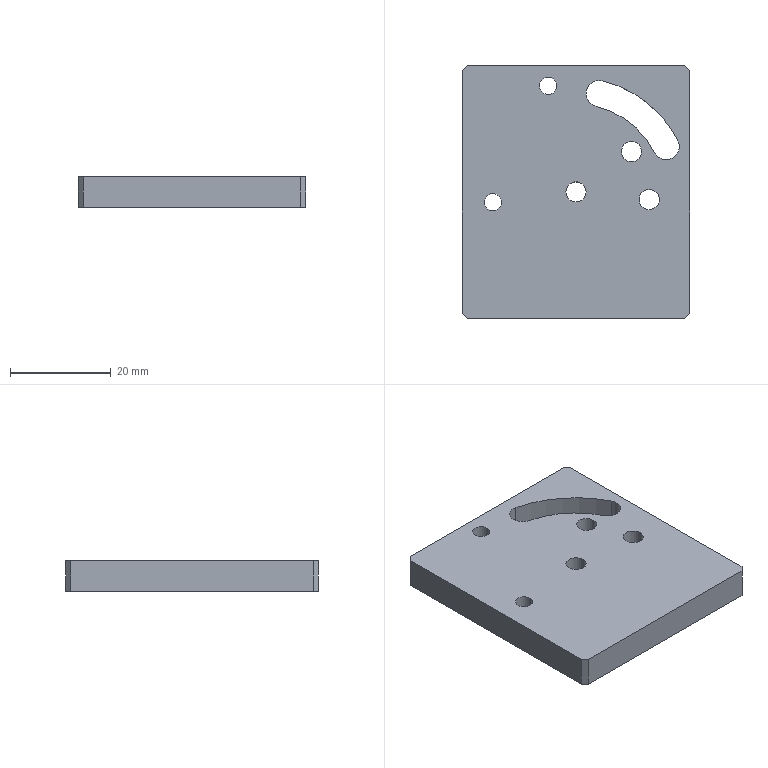Part | NX | features BREP 1 | 1 solid | 31 faces | box 45 x 50 x 6 mm | volume 12312 mm3 | cylinder 19 | plane 12 | commonest cylinder face diameters 4 x6 3.4 x4 6.5 x4 5.2 x3 34.8 x1 45.2 x1
STEP:
#1=CARTESIAN_POINT('',(12.5,-1.5,6.));
#2=VERTEX_POINT('',#1);
#3=CARTESIAN_POINT('',(16.5,-1.5,6.));
#4=VERTEX_POINT('',#3);
#5=CARTESIAN_POINT('',(14.5,-1.5,6.));
#6=DIRECTION('',(0.,0.,1.));
#7=DIRECTION('',(1.,0.,0.));
#8=AXIS2_PLACEMENT_3D('',#5,#6,#7);
#9=CIRCLE('',#8,2.);
#10=EDGE_CURVE('',#2,#4,#9,.T.);
#11=ORIENTED_EDGE('',*,*,#10,.T.);
#12=CARTESIAN_POINT('',(16.5,-1.5,0.));
#13=VERTEX_POINT('',#12);
#14=CARTESIAN_POINT('',(16.5,-1.5,10.));
#15=DIRECTION('',(0.,0.,-1.));
#16=VECTOR('',#15,1000.);
#17=LINE('',#14,#16);
#18=EDGE_CURVE('',#4,#13,#17,.T.);
#19=ORIENTED_EDGE('',*,*,#18,.T.);
#20=CARTESIAN_POINT('',(12.5,-1.5,0.));
#21=VERTEX_POINT('',#20);
#22=CARTESIAN_POINT('',(14.5,-1.5,0.));
#23=DIRECTION('',(0.,0.,-1.));
#24=DIRECTION('',(-1.,0.,0.));
#25=AXIS2_PLACEMENT_3D('',#22,#23,#24);
#26=CIRCLE('',#25,2.);
#27=EDGE_CURVE('',#13,#21,#26,.T.);
#28=ORIENTED_EDGE('',*,*,#27,.T.);
#29=CARTESIAN_POINT('',(12.5,-1.5,10.));
#30=DIRECTION('',(0.,0.,-1.));
#31=VECTOR('',#30,1000.);
#32=LINE('',#29,#31);
#33=EDGE_CURVE('',#2,#21,#32,.T.);
#34=ORIENTED_EDGE('',*,*,#33,.F.);
#35=EDGE_LOOP('',(#11,#19,#28,#34));
#36=FACE_BOUND('',#35,.T.);
#37=CARTESIAN_POINT('',(14.5,-1.5,10.));
#38=DIRECTION('',(0.,0.,-1.));
#39=DIRECTION('',(-1.,0.,0.));
#40=AXIS2_PLACEMENT_3D('',#37,#38,#39);
#41=CYLINDRICAL_SURFACE('',#40,2.);
#42=ADVANCED_FACE('',(#36),#41,.F.);
#43=CARTESIAN_POINT('',(9.,8.,6.));
#44=VERTEX_POINT('',#43);
#45=CARTESIAN_POINT('',(13.,8.,6.));
#46=VERTEX_POINT('',#45);
#47=CARTESIAN_POINT('',(11.,8.,6.));
#48=DIRECTION('',(0.,0.,1.));
#49=DIRECTION('',(1.,0.,0.));
#50=AXIS2_PLACEMENT_3D('',#47,#48,#49);
#51=CIRCLE('',#50,2.);
#52=EDGE_CURVE('',#44,#46,#51,.T.);
#53=ORIENTED_EDGE('',*,*,#52,.T.);
#54=CARTESIAN_POINT('',(13.,8.,0.));
#55=VERTEX_POINT('',#54);
#56=CARTESIAN_POINT('',(13.,8.,10.));
#57=DIRECTION('',(0.,0.,-1.));
#58=VECTOR('',#57,1000.);
#59=LINE('',#56,#58);
#60=EDGE_CURVE('',#46,#55,#59,.T.);
#61=ORIENTED_EDGE('',*,*,#60,.T.);
#62=CARTESIAN_POINT('',(9.,8.,0.));
#63=VERTEX_POINT('',#62);
#64=CARTESIAN_POINT('',(11.,8.,0.));
#65=DIRECTION('',(0.,0.,-1.));
#66=DIRECTION('',(-1.,0.,0.));
#67=AXIS2_PLACEMENT_3D('',#64,#65,#66);
#68=CIRCLE('',#67,2.);
#69=EDGE_CURVE('',#55,#63,#68,.T.);
#70=ORIENTED_EDGE('',*,*,#69,.T.);
#71=CARTESIAN_POINT('',(9.,8.,10.));
#72=DIRECTION('',(0.,0.,-1.));
#73=VECTOR('',#72,1000.);
#74=LINE('',#71,#73);
#75=EDGE_CURVE('',#44,#63,#74,.T.);
#76=ORIENTED_EDGE('',*,*,#75,.F.);
#77=EDGE_LOOP('',(#53,#61,#70,#76));
#78=FACE_BOUND('',#77,.T.);
#79=CARTESIAN_POINT('',(11.,8.,10.));
#80=DIRECTION('',(0.,0.,-1.));
#81=DIRECTION('',(-1.,0.,0.));
#82=AXIS2_PLACEMENT_3D('',#79,#80,#81);
#83=CYLINDRICAL_SURFACE('',#82,2.);
#84=ADVANCED_FACE('',(#78),#83,.F.);
#85=CARTESIAN_POINT('',(-13.25,-2.,3.5));
#86=VERTEX_POINT('',#85);
#87=CARTESIAN_POINT('',(-19.75,-2.,3.5));
#88=VERTEX_POINT('',#87);
#89=CARTESIAN_POINT('',(-16.5,-2.,3.5));
#90=DIRECTION('',(0.,0.,-1.));
#91=DIRECTION('',(-1.,0.,0.));
#92=AXIS2_PLACEMENT_3D('',#89,#90,#91);
#93=CIRCLE('',#92,3.25);
#94=EDGE_CURVE('',#86,#88,#93,.T.);
#95=ORIENTED_EDGE('',*,*,#94,.F.);
#96=CARTESIAN_POINT('',(-13.25,-2.,0.));
#97=VERTEX_POINT('',#96);
#98=CARTESIAN_POINT('',(-13.25,-2.,0.));
#99=DIRECTION('',(0.,0.,-1.));
#100=VECTOR('',#99,1000.);
#101=LINE('',#98,#100);
#102=EDGE_CURVE('',#86,#97,#101,.T.);
#103=ORIENTED_EDGE('',*,*,#102,.T.);
#104=CARTESIAN_POINT('',(-19.75,-2.,0.));
#105=VERTEX_POINT('',#104);
#106=CARTESIAN_POINT('',(-16.5,-2.,0.));
#107=DIRECTION('',(0.,0.,-1.));
#108=DIRECTION('',(-1.,0.,0.));
#109=AXIS2_PLACEMENT_3D('',#106,#107,#108);
#110=CIRCLE('',#109,3.25);
#111=EDGE_CURVE('',#97,#105,#110,.T.);
#112=ORIENTED_EDGE('',*,*,#111,.T.);
#113=CARTESIAN_POINT('',(-19.75,-2.,0.));
#114=DIRECTION('',(0.,0.,-1.));
#115=VECTOR('',#114,1000.);
#116=LINE('',#113,#115);
#117=EDGE_CURVE('',#88,#105,#116,.T.);
#118=ORIENTED_EDGE('',*,*,#117,.F.);
#119=EDGE_LOOP('',(#95,#103,#112,#118));
#120=FACE_BOUND('',#119,.T.);
#121=CARTESIAN_POINT('',(-16.5,-2.,0.));
#122=DIRECTION('',(0.,0.,-1.));
#123=DIRECTION('',(-1.,0.,0.));
#124=AXIS2_PLACEMENT_3D('',#121,#122,#123);
#125=CYLINDRICAL_SURFACE('',#124,3.25);
#126=ADVANCED_FACE('',(#120),#125,.F.);
#127=CARTESIAN_POINT('',(-14.8,-2.,6.));
#128=VERTEX_POINT('',#127);
#129=CARTESIAN_POINT('',(-18.2,-2.,6.));
#130=VERTEX_POINT('',#129);
#131=CARTESIAN_POINT('',(-16.5,-2.,6.));
#132=DIRECTION('',(0.,0.,-1.));
#133=DIRECTION('',(-1.,0.,0.));
#134=AXIS2_PLACEMENT_3D('',#131,#132,#133);
#135=CIRCLE('',#134,1.7);
#136=EDGE_CURVE('',#128,#130,#135,.T.);
#137=ORIENTED_EDGE('',*,*,#136,.F.);
#138=CARTESIAN_POINT('',(-14.8,-2.,3.5));
#139=VERTEX_POINT('',#138);
#140=CARTESIAN_POINT('',(-14.8,-2.,0.));
#141=DIRECTION('',(0.,0.,-1.));
#142=VECTOR('',#141,1000.);
#143=LINE('',#140,#142);
#144=EDGE_CURVE('',#128,#139,#143,.T.);
#145=ORIENTED_EDGE('',*,*,#144,.T.);
#146=CARTESIAN_POINT('',(-18.2,-2.,3.5));
#147=VERTEX_POINT('',#146);
#148=CARTESIAN_POINT('',(-16.5,-2.,3.5));
#149=DIRECTION('',(0.,0.,-1.));
#150=DIRECTION('',(-1.,0.,0.));
#151=AXIS2_PLACEMENT_3D('',#148,#149,#150);
#152=CIRCLE('',#151,1.7);
#153=EDGE_CURVE('',#139,#147,#152,.T.);
#154=ORIENTED_EDGE('',*,*,#153,.T.);
#155=CARTESIAN_POINT('',(-18.2,-2.,0.));
#156=DIRECTION('',(0.,0.,-1.));
#157=VECTOR('',#156,1000.);
#158=LINE('',#155,#157);
#159=EDGE_CURVE('',#130,#147,#158,.T.);
#160=ORIENTED_EDGE('',*,*,#159,.F.);
#161=EDGE_LOOP('',(#137,#145,#154,#160));
#162=FACE_BOUND('',#161,.T.);
#163=CARTESIAN_POINT('',(-16.5,-2.,0.));
#164=DIRECTION('',(0.,0.,-1.));
#165=DIRECTION('',(-1.,0.,0.));
#166=AXIS2_PLACEMENT_3D('',#163,#164,#165);
#167=CYLINDRICAL_SURFACE('',#166,1.7);
#168=ADVANCED_FACE('',(#162),#167,.F.);
#169=CARTESIAN_POINT('',(-2.25,21.,3.5));
#170=VERTEX_POINT('',#169);
#171=CARTESIAN_POINT('',(-8.75,21.,3.5));
#172=VERTEX_POINT('',#171);
#173=CARTESIAN_POINT('',(-5.5,21.,3.5));
#174=DIRECTION('',(0.,0.,-1.));
#175=DIRECTION('',(-1.,0.,0.));
#176=AXIS2_PLACEMENT_3D('',#173,#174,#175);
#177=CIRCLE('',#176,3.25);
#178=EDGE_CURVE('',#170,#172,#177,.T.);
#179=ORIENTED_EDGE('',*,*,#178,.F.);
#180=CARTESIAN_POINT('',(-2.25,21.,0.));
#181=VERTEX_POINT('',#180);
#182=CARTESIAN_POINT('',(-2.25,21.,0.));
#183=DIRECTION('',(0.,0.,-1.));
#184=VECTOR('',#183,1000.);
#185=LINE('',#182,#184);
#186=EDGE_CURVE('',#170,#181,#185,.T.);
#187=ORIENTED_EDGE('',*,*,#186,.T.);
#188=CARTESIAN_POINT('',(-8.75,21.,0.));
#189=VERTEX_POINT('',#188);
#190=CARTESIAN_POINT('',(-5.5,21.,0.));
#191=DIRECTION('',(0.,0.,-1.));
#192=DIRECTION('',(-1.,0.,0.));
#193=AXIS2_PLACEMENT_3D('',#190,#191,#192);
#194=CIRCLE('',#193,3.25);
#195=EDGE_CURVE('',#181,#189,#194,.T.);
#196=ORIENTED_EDGE('',*,*,#195,.T.);
#197=CARTESIAN_POINT('',(-8.75,21.,0.));
#198=DIRECTION('',(0.,0.,-1.));
#199=VECTOR('',#198,1000.);
#200=LINE('',#197,#199);
#201=EDGE_CURVE('',#172,#189,#200,.T.);
#202=ORIENTED_EDGE('',*,*,#201,.F.);
#203=EDGE_LOOP('',(#179,#187,#196,#202));
#204=FACE_BOUND('',#203,.T.);
#205=CARTESIAN_POINT('',(-5.5,21.,0.));
#206=DIRECTION('',(0.,0.,-1.));
#207=DIRECTION('',(-1.,0.,0.));
#208=AXIS2_PLACEMENT_3D('',#205,#206,#207);
#209=CYLINDRICAL_SURFACE('',#208,3.25);
#210=ADVANCED_FACE('',(#204),#209,.F.);
#211=CARTESIAN_POINT('',(-3.8,21.,6.));
#212=VERTEX_POINT('',#211);
#213=CARTESIAN_POINT('',(-7.2,21.,6.));
#214=VERTEX_POINT('',#213);
#215=CARTESIAN_POINT('',(-5.5,21.,6.));
#216=DIRECTION('',(0.,0.,-1.));
#217=DIRECTION('',(-1.,0.,0.));
#218=AXIS2_PLACEMENT_3D('',#215,#216,#217);
#219=CIRCLE('',#218,1.7);
#220=EDGE_CURVE('',#212,#214,#219,.T.);
#221=ORIENTED_EDGE('',*,*,#220,.F.);
#222=CARTESIAN_POINT('',(-3.8,21.,3.5));
#223=VERTEX_POINT('',#222);
#224=CARTESIAN_POINT('',(-3.8,21.,0.));
#225=DIRECTION('',(0.,0.,-1.));
#226=VECTOR('',#225,1000.);
#227=LINE('',#224,#226);
#228=EDGE_CURVE('',#212,#223,#227,.T.);
#229=ORIENTED_EDGE('',*,*,#228,.T.);
#230=CARTESIAN_POINT('',(-7.2,21.,3.5));
#231=VERTEX_POINT('',#230);
#232=CARTESIAN_POINT('',(-5.5,21.,3.5));
#233=DIRECTION('',(0.,0.,-1.));
#234=DIRECTION('',(-1.,0.,0.));
#235=AXIS2_PLACEMENT_3D('',#232,#233,#234);
#236=CIRCLE('',#235,1.7);
#237=EDGE_CURVE('',#223,#231,#236,.T.);
#238=ORIENTED_EDGE('',*,*,#237,.T.);
#239=CARTESIAN_POINT('',(-7.2,21.,0.));
#240=DIRECTION('',(0.,0.,-1.));
#241=VECTOR('',#240,1000.);
#242=LINE('',#239,#241);
#243=EDGE_CURVE('',#214,#231,#242,.T.);
#244=ORIENTED_EDGE('',*,*,#243,.F.);
#245=EDGE_LOOP('',(#221,#229,#238,#244));
#246=FACE_BOUND('',#245,.T.);
#247=CARTESIAN_POINT('',(-5.5,21.,0.));
#248=DIRECTION('',(0.,0.,-1.));
#249=DIRECTION('',(-1.,0.,0.));
#250=AXIS2_PLACEMENT_3D('',#247,#248,#249);
#251=CYLINDRICAL_SURFACE('',#250,1.7);
#252=ADVANCED_FACE('',(#246),#251,.F.);
#253=CARTESIAN_POINT('',(5.182,21.998,6.));
#254=VERTEX_POINT('',#253);
#255=CARTESIAN_POINT('',(1.986,19.467,6.));
#256=VERTEX_POINT('',#255);
#257=CARTESIAN_POINT('',(4.586,19.467,6.));
#258=DIRECTION('',(0.,0.,1.));
#259=DIRECTION('',(1.,0.,0.));
#260=AXIS2_PLACEMENT_3D('',#257,#258,#259);
#261=CIRCLE('',#260,2.6);
#262=EDGE_CURVE('',#254,#256,#261,.T.);
#263=ORIENTED_EDGE('',*,*,#262,.T.);
#264=CARTESIAN_POINT('',(1.986,19.467,0.));
#265=VERTEX_POINT('',#264);
#266=CARTESIAN_POINT('',(1.986,19.467,10.));
#267=DIRECTION('',(0.,0.,-1.));
#268=VECTOR('',#267,1000.);
#269=LINE('',#266,#268);
#270=EDGE_CURVE('',#256,#265,#269,.T.);
#271=ORIENTED_EDGE('',*,*,#270,.T.);
#272=CARTESIAN_POINT('',(5.182,21.998,0.));
#273=VERTEX_POINT('',#272);
#274=CARTESIAN_POINT('',(4.586,19.467,0.));
#275=DIRECTION('',(0.,0.,-1.));
#276=DIRECTION('',(-1.,0.,0.));
#277=AXIS2_PLACEMENT_3D('',#274,#275,#276);
#278=CIRCLE('',#277,2.6);
#279=EDGE_CURVE('',#265,#273,#278,.T.);
#280=ORIENTED_EDGE('',*,*,#279,.T.);
#281=CARTESIAN_POINT('',(5.182,21.998,10.));
#282=DIRECTION('',(0.,0.,-1.));
#283=VECTOR('',#282,1000.);
#284=LINE('',#281,#283);
#285=EDGE_CURVE('',#254,#273,#284,.T.);
#286=ORIENTED_EDGE('',*,*,#285,.F.);
#287=EDGE_LOOP('',(#263,#271,#280,#286));
#288=FACE_BOUND('',#287,.T.);
#289=CARTESIAN_POINT('',(4.586,19.467,10.));
#290=DIRECTION('',(0.,0.,-1.));
#291=DIRECTION('',(-1.,0.,0.));
#292=AXIS2_PLACEMENT_3D('',#289,#290,#291);
#293=CYLINDRICAL_SURFACE('',#292,2.6);
#294=ADVANCED_FACE('',(#288),#293,.F.);
#295=CARTESIAN_POINT('',(-2.,0.,6.));
#296=VERTEX_POINT('',#295);
#297=CARTESIAN_POINT('',(2.,0.,6.));
#298=VERTEX_POINT('',#297);
#299=CARTESIAN_POINT('',(0.,0.,6.));
#300=DIRECTION('',(0.,0.,1.));
#301=DIRECTION('',(1.,0.,0.));
#302=AXIS2_PLACEMENT_3D('',#299,#300,#301);
#303=CIRCLE('',#302,2.);
#304=EDGE_CURVE('',#296,#298,#303,.T.);
#305=ORIENTED_EDGE('',*,*,#304,.T.);
#306=CARTESIAN_POINT('',(2.,0.,0.));
#307=VERTEX_POINT('',#306);
#308=CARTESIAN_POINT('',(2.,0.,10.));
#309=DIRECTION('',(0.,0.,-1.));
#310=VECTOR('',#309,1000.);
#311=LINE('',#308,#310);
#312=EDGE_CURVE('',#298,#307,#311,.T.);
#313=ORIENTED_EDGE('',*,*,#312,.T.);
#314=CARTESIAN_POINT('',(-2.,0.,0.));
#315=VERTEX_POINT('',#314);
#316=CARTESIAN_POINT('',(0.,0.,0.));
#317=DIRECTION('',(0.,0.,-1.));
#318=DIRECTION('',(-1.,0.,0.));
#319=AXIS2_PLACEMENT_3D('',#316,#317,#318);
#320=CIRCLE('',#319,2.);
#321=EDGE_CURVE('',#307,#315,#320,.T.);
#322=ORIENTED_EDGE('',*,*,#321,.T.);
#323=CARTESIAN_POINT('',(-2.,0.,10.));
#324=DIRECTION('',(0.,0.,-1.));
#325=VECTOR('',#324,1000.);
#326=LINE('',#323,#325);
#327=EDGE_CURVE('',#296,#315,#326,.T.);
#328=ORIENTED_EDGE('',*,*,#327,.F.);
#329=EDGE_LOOP('',(#305,#313,#322,#328));
#330=FACE_BOUND('',#329,.T.);
#331=CARTESIAN_POINT('',(0.,0.,10.));
#332=DIRECTION('',(0.,0.,-1.));
#333=DIRECTION('',(-1.,0.,0.));
#334=AXIS2_PLACEMENT_3D('',#331,#332,#333);
#335=CYLINDRICAL_SURFACE('',#334,2.);
#336=ADVANCED_FACE('',(#330),#335,.F.);
#337=CARTESIAN_POINT('',(22.5,-24.,6.));
#338=VERTEX_POINT('',#337);
#339=CARTESIAN_POINT('',(22.5,24.,6.));
#340=VERTEX_POINT('',#339);
#341=CARTESIAN_POINT('',(22.5,25.,6.));
#342=DIRECTION('',(0.,1.,0.));
#343=VECTOR('',#342,1000.);
#344=LINE('',#341,#343);
#345=EDGE_CURVE('',#338,#340,#344,.T.);
#346=ORIENTED_EDGE('',*,*,#345,.F.);
#347=CARTESIAN_POINT('',(22.5,-24.,0.));
#348=VERTEX_POINT('',#347);
#349=CARTESIAN_POINT('',(22.5,-24.,6.));
#350=DIRECTION('',(0.,0.,-1.));
#351=VECTOR('',#350,1000.);
#352=LINE('',#349,#351);
#353=EDGE_CURVE('',#338,#348,#352,.T.);
#354=ORIENTED_EDGE('',*,*,#353,.T.);
#355=CARTESIAN_POINT('',(22.5,24.,0.));
#356=VERTEX_POINT('',#355);
#357=CARTESIAN_POINT('',(22.5,25.,0.));
#358=DIRECTION('',(0.,1.,0.));
#359=VECTOR('',#358,1000.);
#360=LINE('',#357,#359);
#361=EDGE_CURVE('',#348,#356,#360,.T.);
#362=ORIENTED_EDGE('',*,*,#361,.T.);
#363=CARTESIAN_POINT('',(22.5,24.,6.));
#364=DIRECTION('',(0.,0.,1.));
#365=VECTOR('',#364,1000.);
#366=LINE('',#363,#365);
#367=EDGE_CURVE('',#356,#340,#366,.T.);
#368=ORIENTED_EDGE('',*,*,#367,.T.);
#369=EDGE_LOOP('',(#346,#354,#362,#368));
#370=FACE_BOUND('',#369,.T.);
#371=CARTESIAN_POINT('',(22.5,25.,6.));
#372=DIRECTION('',(-1.,0.,0.));
#373=DIRECTION('',(0.,1.,0.));
#374=AXIS2_PLACEMENT_3D('',#371,#372,#373);
#375=PLANE('',#374);
#376=ADVANCED_FACE('',(#370),#375,.F.);
#377=CARTESIAN_POINT('',(21.5,25.,0.));
#378=VERTEX_POINT('',#377);
#379=CARTESIAN_POINT('',(-21.5,25.,0.));
#380=VERTEX_POINT('',#379);
#381=CARTESIAN_POINT('',(-22.5,25.,0.));
#382=DIRECTION('',(-1.,0.,0.));
#383=VECTOR('',#382,1000.);
#384=LINE('',#381,#383);
#385=EDGE_CURVE('',#378,#380,#384,.T.);
#386=ORIENTED_EDGE('',*,*,#385,.T.);
#387=CARTESIAN_POINT('',(-21.5,25.,6.));
#388=VERTEX_POINT('',#387);
#389=CARTESIAN_POINT('',(-21.5,25.,6.));
#390=DIRECTION('',(0.,0.,1.));
#391=VECTOR('',#390,1000.);
#392=LINE('',#389,#391);
#393=EDGE_CURVE('',#380,#388,#392,.T.);
#394=ORIENTED_EDGE('',*,*,#393,.T.);
#395=CARTESIAN_POINT('',(21.5,25.,6.));
#396=VERTEX_POINT('',#395);
#397=CARTESIAN_POINT('',(-22.5,25.,6.));
#398=DIRECTION('',(-1.,0.,0.));
#399=VECTOR('',#398,1000.);
#400=LINE('',#397,#399);
#401=EDGE_CURVE('',#396,#388,#400,.T.);
#402=ORIENTED_EDGE('',*,*,#401,.F.);
#403=CARTESIAN_POINT('',(21.5,25.,6.));
#404=DIRECTION('',(0.,0.,-1.));
#405=VECTOR('',#404,1000.);
#406=LINE('',#403,#405);
#407=EDGE_CURVE('',#396,#378,#406,.T.);
#408=ORIENTED_EDGE('',*,*,#407,.T.);
#409=EDGE_LOOP('',(#386,#394,#402,#408));
#410=FACE_BOUND('',#409,.T.);
#411=CARTESIAN_POINT('',(-22.5,25.,6.));
#412=DIRECTION('',(0.,-1.,0.));
#413=DIRECTION('',(0.,0.,-1.));
#414=AXIS2_PLACEMENT_3D('',#411,#412,#413);
#415=PLANE('',#414);
#416=ADVANCED_FACE('',(#410),#415,.F.);
#417=CARTESIAN_POINT('',(-22.5,24.,0.));
#418=VERTEX_POINT('',#417);
#419=CARTESIAN_POINT('',(-22.5,-24.,0.));
#420=VERTEX_POINT('',#419);
#421=CARTESIAN_POINT('',(-22.5,25.,0.));
#422=DIRECTION('',(0.,-1.,0.));
#423=VECTOR('',#422,1000.);
#424=LINE('',#421,#423);
#425=EDGE_CURVE('',#418,#420,#424,.T.);
#426=ORIENTED_EDGE('',*,*,#425,.T.);
#427=CARTESIAN_POINT('',(-22.5,-24.,6.));
#428=VERTEX_POINT('',#427);
#429=CARTESIAN_POINT('',(-22.5,-24.,6.));
#430=DIRECTION('',(0.,0.,1.));
#431=VECTOR('',#430,1000.);
#432=LINE('',#429,#431);
#433=EDGE_CURVE('',#420,#428,#432,.T.);
#434=ORIENTED_EDGE('',*,*,#433,.T.);
#435=CARTESIAN_POINT('',(-22.5,24.,6.));
#436=VERTEX_POINT('',#435);
#437=CARTESIAN_POINT('',(-22.5,25.,6.));
#438=DIRECTION('',(0.,-1.,0.));
#439=VECTOR('',#438,1000.);
#440=LINE('',#437,#439);
#441=EDGE_CURVE('',#436,#428,#440,.T.);
#442=ORIENTED_EDGE('',*,*,#441,.F.);
#443=CARTESIAN_POINT('',(-22.5,24.,6.));
#444=DIRECTION('',(0.,0.,-1.));
#445=VECTOR('',#444,1000.);
#446=LINE('',#443,#445);
#447=EDGE_CURVE('',#436,#418,#446,.T.);
#448=ORIENTED_EDGE('',*,*,#447,.T.);
#449=EDGE_LOOP('',(#426,#434,#442,#448));
#450=FACE_BOUND('',#449,.T.);
#451=CARTESIAN_POINT('',(-22.5,25.,6.));
#452=DIRECTION('',(1.,0.,0.));
#453=DIRECTION('',(0.,1.,0.));
#454=AXIS2_PLACEMENT_3D('',#451,#452,#453);
#455=PLANE('',#454);
#456=ADVANCED_FACE('',(#450),#455,.F.);
#457=CARTESIAN_POINT('',(-21.5,-25.,6.));
#458=VERTEX_POINT('',#457);
#459=CARTESIAN_POINT('',(21.5,-25.,6.));
#460=VERTEX_POINT('',#459);
#461=CARTESIAN_POINT('',(-22.5,-25.,6.));
#462=DIRECTION('',(1.,0.,0.));
#463=VECTOR('',#462,1000.);
#464=LINE('',#461,#463);
#465=EDGE_CURVE('',#458,#460,#464,.T.);
#466=ORIENTED_EDGE('',*,*,#465,.F.);
#467=CARTESIAN_POINT('',(-21.5,-25.,0.));
#468=VERTEX_POINT('',#467);
#469=CARTESIAN_POINT('',(-21.5,-25.,6.));
#470=DIRECTION('',(0.,0.,-1.));
#471=VECTOR('',#470,1000.);
#472=LINE('',#469,#471);
#473=EDGE_CURVE('',#458,#468,#472,.T.);
#474=ORIENTED_EDGE('',*,*,#473,.T.);
#475=CARTESIAN_POINT('',(21.5,-25.,0.));
#476=VERTEX_POINT('',#475);
#477=CARTESIAN_POINT('',(-22.5,-25.,0.));
#478=DIRECTION('',(1.,0.,0.));
#479=VECTOR('',#478,1000.);
#480=LINE('',#477,#479);
#481=EDGE_CURVE('',#468,#476,#480,.T.);
#482=ORIENTED_EDGE('',*,*,#481,.T.);
#483=CARTESIAN_POINT('',(21.5,-25.,6.));
#484=DIRECTION('',(0.,0.,1.));
#485=VECTOR('',#484,1000.);
#486=LINE('',#483,#485);
#487=EDGE_CURVE('',#476,#460,#486,.T.);
#488=ORIENTED_EDGE('',*,*,#487,.T.);
#489=EDGE_LOOP('',(#466,#474,#482,#488));
#490=FACE_BOUND('',#489,.T.);
#491=CARTESIAN_POINT('',(-22.5,-25.,6.));
#492=DIRECTION('',(0.,1.,0.));
#493=DIRECTION('',(1.,0.,0.));
#494=AXIS2_PLACEMENT_3D('',#491,#492,#493);
#495=PLANE('',#494);
#496=ADVANCED_FACE('',(#490),#495,.F.);
#497=ORIENTED_EDGE('',*,*,#441,.T.);
#498=CARTESIAN_POINT('',(-23.25,-23.25,6.));
#499=DIRECTION('',(0.7071,-0.7071,0.));
#500=VECTOR('',#499,1000.);
#501=LINE('',#498,#500);
#502=EDGE_CURVE('',#428,#458,#501,.T.);
#503=ORIENTED_EDGE('',*,*,#502,.T.);
#504=ORIENTED_EDGE('',*,*,#465,.T.);
#505=CARTESIAN_POINT('',(23.25,-23.25,6.));
#506=DIRECTION('',(0.7071,0.7071,0.));
#507=VECTOR('',#506,1000.);
#508=LINE('',#505,#507);
#509=EDGE_CURVE('',#460,#338,#508,.T.);
#510=ORIENTED_EDGE('',*,*,#509,.T.);
#511=ORIENTED_EDGE('',*,*,#345,.T.);
#512=CARTESIAN_POINT('',(23.25,23.25,6.));
#513=DIRECTION('',(-0.7071,0.7071,0.));
#514=VECTOR('',#513,1000.);
#515=LINE('',#512,#514);
#516=EDGE_CURVE('',#340,#396,#515,.T.);
#517=ORIENTED_EDGE('',*,*,#516,.T.);
#518=ORIENTED_EDGE('',*,*,#401,.T.);
#519=CARTESIAN_POINT('',(-23.25,23.25,6.));
#520=DIRECTION('',(-0.7071,-0.7071,0.));
#521=VECTOR('',#520,1000.);
#522=LINE('',#519,#521);
#523=EDGE_CURVE('',#388,#436,#522,.T.);
#524=ORIENTED_EDGE('',*,*,#523,.T.);
#525=EDGE_LOOP('',(#497,#503,#504,#510,#511,#517,#518,#524));
#526=FACE_BOUND('',#525,.T.);
#527=ORIENTED_EDGE('',*,*,#10,.F.);
#528=CARTESIAN_POINT('',(14.5,-1.5,6.));
#529=DIRECTION('',(0.,0.,1.));
#530=DIRECTION('',(1.,0.,0.));
#531=AXIS2_PLACEMENT_3D('',#528,#529,#530);
#532=CIRCLE('',#531,2.);
#533=EDGE_CURVE('',#4,#2,#532,.T.);
#534=ORIENTED_EDGE('',*,*,#533,.F.);
#535=EDGE_LOOP('',(#527,#534));
#536=FACE_BOUND('',#535,.T.);
#537=ORIENTED_EDGE('',*,*,#52,.F.);
#538=CARTESIAN_POINT('',(11.,8.,6.));
#539=DIRECTION('',(0.,0.,1.));
#540=DIRECTION('',(1.,0.,0.));
#541=AXIS2_PLACEMENT_3D('',#538,#539,#540);
#542=CIRCLE('',#541,2.);
#543=EDGE_CURVE('',#46,#44,#542,.T.);
#544=ORIENTED_EDGE('',*,*,#543,.F.);
#545=EDGE_LOOP('',(#537,#544));
#546=FACE_BOUND('',#545,.T.);
#547=CARTESIAN_POINT('',(-16.5,-2.,6.));
#548=DIRECTION('',(0.,0.,-1.));
#549=DIRECTION('',(-1.,0.,0.));
#550=AXIS2_PLACEMENT_3D('',#547,#548,#549);
#551=CIRCLE('',#550,1.7);
#552=EDGE_CURVE('',#130,#128,#551,.T.);
#553=ORIENTED_EDGE('',*,*,#552,.T.);
#554=ORIENTED_EDGE('',*,*,#136,.T.);
#555=EDGE_LOOP('',(#553,#554));
#556=FACE_BOUND('',#555,.T.);
#557=CARTESIAN_POINT('',(-5.5,21.,6.));
#558=DIRECTION('',(0.,0.,-1.));
#559=DIRECTION('',(-1.,0.,0.));
#560=AXIS2_PLACEMENT_3D('',#557,#558,#559);
#561=CIRCLE('',#560,1.7);
#562=EDGE_CURVE('',#214,#212,#561,.T.);
#563=ORIENTED_EDGE('',*,*,#562,.T.);
#564=ORIENTED_EDGE('',*,*,#220,.T.);
#565=EDGE_LOOP('',(#563,#564));
#566=FACE_BOUND('',#565,.T.);
#567=ORIENTED_EDGE('',*,*,#262,.F.);
#568=CARTESIAN_POINT('',(20.182,10.17,6.));
#569=VERTEX_POINT('',#568);
#570=CARTESIAN_POINT('',(0.,0.,6.));
#571=DIRECTION('',(0.,0.,1.));
#572=DIRECTION('',(1.,0.,0.));
#573=AXIS2_PLACEMENT_3D('',#570,#571,#572);
#574=CIRCLE('',#573,22.6);
#575=EDGE_CURVE('',#569,#254,#574,.T.);
#576=ORIENTED_EDGE('',*,*,#575,.F.);
#577=CARTESIAN_POINT('',(15.539,7.83,6.));
#578=VERTEX_POINT('',#577);
#579=CARTESIAN_POINT('',(17.861,9.,6.));
#580=DIRECTION('',(0.,0.,1.));
#581=DIRECTION('',(1.,0.,0.));
#582=AXIS2_PLACEMENT_3D('',#579,#580,#581);
#583=CIRCLE('',#582,2.6);
#584=EDGE_CURVE('',#578,#569,#583,.T.);
#585=ORIENTED_EDGE('',*,*,#584,.F.);
#586=CARTESIAN_POINT('',(3.99,16.936,6.));
#587=VERTEX_POINT('',#586);
#588=CARTESIAN_POINT('',(0.,0.,6.));
#589=DIRECTION('',(0.,0.,-1.));
#590=DIRECTION('',(1.,0.,0.));
#591=AXIS2_PLACEMENT_3D('',#588,#589,#590);
#592=CIRCLE('',#591,17.4);
#593=EDGE_CURVE('',#587,#578,#592,.T.);
#594=ORIENTED_EDGE('',*,*,#593,.F.);
#595=CARTESIAN_POINT('',(4.586,19.467,6.));
#596=DIRECTION('',(0.,0.,1.));
#597=DIRECTION('',(1.,0.,0.));
#598=AXIS2_PLACEMENT_3D('',#595,#596,#597);
#599=CIRCLE('',#598,2.6);
#600=EDGE_CURVE('',#256,#587,#599,.T.);
#601=ORIENTED_EDGE('',*,*,#600,.F.);
#602=EDGE_LOOP('',(#567,#576,#585,#594,#601));
#603=FACE_BOUND('',#602,.T.);
#604=ORIENTED_EDGE('',*,*,#304,.F.);
#605=CARTESIAN_POINT('',(0.,0.,6.));
#606=DIRECTION('',(0.,0.,1.));
#607=DIRECTION('',(1.,0.,0.));
#608=AXIS2_PLACEMENT_3D('',#605,#606,#607);
#609=CIRCLE('',#608,2.);
#610=EDGE_CURVE('',#298,#296,#609,.T.);
#611=ORIENTED_EDGE('',*,*,#610,.F.);
#612=EDGE_LOOP('',(#604,#611));
#613=FACE_BOUND('',#612,.T.);
#614=CARTESIAN_POINT('',(0.,0.,6.));
#615=DIRECTION('',(0.,0.,1.));
#616=DIRECTION('',(1.,0.,0.));
#617=AXIS2_PLACEMENT_3D('',#614,#615,#616);
#618=PLANE('',#617);
#619=ADVANCED_FACE('',(#526,#536,#546,#556,#566,#603,#613),#618,.T.);
#620=ORIENTED_EDGE('',*,*,#481,.F.);
#621=CARTESIAN_POINT('',(-21.5,-25.,0.));
#622=DIRECTION('',(-0.7071,0.7071,0.));
#623=VECTOR('',#622,1000.);
#624=LINE('',#621,#623);
#625=EDGE_CURVE('',#468,#420,#624,.T.);
#626=ORIENTED_EDGE('',*,*,#625,.T.);
#627=ORIENTED_EDGE('',*,*,#425,.F.);
#628=CARTESIAN_POINT('',(-22.5,24.,0.));
#629=DIRECTION('',(0.7071,0.7071,0.));
#630=VECTOR('',#629,1000.);
#631=LINE('',#628,#630);
#632=EDGE_CURVE('',#418,#380,#631,.T.);
#633=ORIENTED_EDGE('',*,*,#632,.T.);
#634=ORIENTED_EDGE('',*,*,#385,.F.);
#635=CARTESIAN_POINT('',(21.5,25.,0.));
#636=DIRECTION('',(0.7071,-0.7071,0.));
#637=VECTOR('',#636,1000.);
#638=LINE('',#635,#637);
#639=EDGE_CURVE('',#378,#356,#638,.T.);
#640=ORIENTED_EDGE('',*,*,#639,.T.);
#641=ORIENTED_EDGE('',*,*,#361,.F.);
#642=CARTESIAN_POINT('',(22.5,-24.,0.));
#643=DIRECTION('',(-0.7071,-0.7071,0.));
#644=VECTOR('',#643,1000.);
#645=LINE('',#642,#644);
#646=EDGE_CURVE('',#348,#476,#645,.T.);
#647=ORIENTED_EDGE('',*,*,#646,.T.);
#648=EDGE_LOOP('',(#620,#626,#627,#633,#634,#640,#641,#647));
#649=FACE_BOUND('',#648,.T.);
#650=CARTESIAN_POINT('',(14.5,-1.5,0.));
#651=DIRECTION('',(0.,0.,-1.));
#652=DIRECTION('',(-1.,0.,0.));
#653=AXIS2_PLACEMENT_3D('',#650,#651,#652);
#654=CIRCLE('',#653,2.);
#655=EDGE_CURVE('',#21,#13,#654,.T.);
#656=ORIENTED_EDGE('',*,*,#655,.F.);
#657=ORIENTED_EDGE('',*,*,#27,.F.);
#658=EDGE_LOOP('',(#656,#657));
#659=FACE_BOUND('',#658,.T.);
#660=CARTESIAN_POINT('',(11.,8.,0.));
#661=DIRECTION('',(0.,0.,-1.));
#662=DIRECTION('',(-1.,0.,0.));
#663=AXIS2_PLACEMENT_3D('',#660,#661,#662);
#664=CIRCLE('',#663,2.);
#665=EDGE_CURVE('',#63,#55,#664,.T.);
#666=ORIENTED_EDGE('',*,*,#665,.F.);
#667=ORIENTED_EDGE('',*,*,#69,.F.);
#668=EDGE_LOOP('',(#666,#667));
#669=FACE_BOUND('',#668,.T.);
#670=CARTESIAN_POINT('',(-16.5,-2.,0.));
#671=DIRECTION('',(0.,0.,-1.));
#672=DIRECTION('',(-1.,0.,0.));
#673=AXIS2_PLACEMENT_3D('',#670,#671,#672);
#674=CIRCLE('',#673,3.25);
#675=EDGE_CURVE('',#105,#97,#674,.T.);
#676=ORIENTED_EDGE('',*,*,#675,.F.);
#677=ORIENTED_EDGE('',*,*,#111,.F.);
#678=EDGE_LOOP('',(#676,#677));
#679=FACE_BOUND('',#678,.T.);
#680=CARTESIAN_POINT('',(-5.5,21.,0.));
#681=DIRECTION('',(0.,0.,-1.));
#682=DIRECTION('',(-1.,0.,0.));
#683=AXIS2_PLACEMENT_3D('',#680,#681,#682);
#684=CIRCLE('',#683,3.25);
#685=EDGE_CURVE('',#189,#181,#684,.T.);
#686=ORIENTED_EDGE('',*,*,#685,.F.);
#687=ORIENTED_EDGE('',*,*,#195,.F.);
#688=EDGE_LOOP('',(#686,#687));
#689=FACE_BOUND('',#688,.T.);
#690=CARTESIAN_POINT('',(20.182,10.17,0.));
#691=VERTEX_POINT('',#690);
#692=CARTESIAN_POINT('',(0.,0.,0.));
#693=DIRECTION('',(0.,0.,-1.));
#694=DIRECTION('',(-1.,0.,0.));
#695=AXIS2_PLACEMENT_3D('',#692,#693,#694);
#696=CIRCLE('',#695,22.6);
#697=EDGE_CURVE('',#273,#691,#696,.T.);
#698=ORIENTED_EDGE('',*,*,#697,.F.);
#699=ORIENTED_EDGE('',*,*,#279,.F.);
#700=CARTESIAN_POINT('',(3.99,16.936,0.));
#701=VERTEX_POINT('',#700);
#702=CARTESIAN_POINT('',(4.586,19.467,0.));
#703=DIRECTION('',(0.,0.,-1.));
#704=DIRECTION('',(-1.,0.,0.));
#705=AXIS2_PLACEMENT_3D('',#702,#703,#704);
#706=CIRCLE('',#705,2.6);
#707=EDGE_CURVE('',#701,#265,#706,.T.);
#708=ORIENTED_EDGE('',*,*,#707,.F.);
#709=CARTESIAN_POINT('',(15.539,7.83,0.));
#710=VERTEX_POINT('',#709);
#711=CARTESIAN_POINT('',(0.,0.,0.));
#712=DIRECTION('',(0.,0.,1.));
#713=DIRECTION('',(-1.,0.,0.));
#714=AXIS2_PLACEMENT_3D('',#711,#712,#713);
#715=CIRCLE('',#714,17.4);
#716=EDGE_CURVE('',#710,#701,#715,.T.);
#717=ORIENTED_EDGE('',*,*,#716,.F.);
#718=CARTESIAN_POINT('',(17.861,9.,0.));
#719=DIRECTION('',(0.,0.,-1.));
#720=DIRECTION('',(-1.,0.,0.));
#721=AXIS2_PLACEMENT_3D('',#718,#719,#720);
#722=CIRCLE('',#721,2.6);
#723=EDGE_CURVE('',#691,#710,#722,.T.);
#724=ORIENTED_EDGE('',*,*,#723,.F.);
#725=EDGE_LOOP('',(#698,#699,#708,#717,#724));
#726=FACE_BOUND('',#725,.T.);
#727=CARTESIAN_POINT('',(0.,0.,0.));
#728=DIRECTION('',(0.,0.,-1.));
#729=DIRECTION('',(-1.,0.,0.));
#730=AXIS2_PLACEMENT_3D('',#727,#728,#729);
#731=CIRCLE('',#730,2.);
#732=EDGE_CURVE('',#315,#307,#731,.T.);
#733=ORIENTED_EDGE('',*,*,#732,.F.);
#734=ORIENTED_EDGE('',*,*,#321,.F.);
#735=EDGE_LOOP('',(#733,#734));
#736=FACE_BOUND('',#735,.T.);
#737=CARTESIAN_POINT('',(0.,0.,0.));
#738=DIRECTION('',(0.,0.,1.));
#739=DIRECTION('',(1.,0.,0.));
#740=AXIS2_PLACEMENT_3D('',#737,#738,#739);
#741=PLANE('',#740);
#742=ADVANCED_FACE('',(#649,#659,#669,#679,#689,#726,#736),#741,.F.);
#743=ORIENTED_EDGE('',*,*,#502,.F.);
#744=ORIENTED_EDGE('',*,*,#433,.F.);
#745=ORIENTED_EDGE('',*,*,#625,.F.);
#746=ORIENTED_EDGE('',*,*,#473,.F.);
#747=EDGE_LOOP('',(#743,#744,#745,#746));
#748=FACE_BOUND('',#747,.T.);
#749=CARTESIAN_POINT('',(-21.5,-25.,6.));
#750=DIRECTION('',(0.7071,0.7071,0.));
#751=DIRECTION('',(0.,0.,-1.));
#752=AXIS2_PLACEMENT_3D('',#749,#750,#751);
#753=PLANE('',#752);
#754=ADVANCED_FACE('',(#748),#753,.F.);
#755=ORIENTED_EDGE('',*,*,#509,.F.);
#756=ORIENTED_EDGE('',*,*,#487,.F.);
#757=ORIENTED_EDGE('',*,*,#646,.F.);
#758=ORIENTED_EDGE('',*,*,#353,.F.);
#759=EDGE_LOOP('',(#755,#756,#757,#758));
#760=FACE_BOUND('',#759,.T.);
#761=CARTESIAN_POINT('',(22.5,-24.,6.));
#762=DIRECTION('',(-0.7071,0.7071,0.));
#763=DIRECTION('',(0.,0.,1.));
#764=AXIS2_PLACEMENT_3D('',#761,#762,#763);
#765=PLANE('',#764);
#766=ADVANCED_FACE('',(#760),#765,.F.);
#767=ORIENTED_EDGE('',*,*,#523,.F.);
#768=ORIENTED_EDGE('',*,*,#393,.F.);
#769=ORIENTED_EDGE('',*,*,#632,.F.);
#770=ORIENTED_EDGE('',*,*,#447,.F.);
#771=EDGE_LOOP('',(#767,#768,#769,#770));
#772=FACE_BOUND('',#771,.T.);
#773=CARTESIAN_POINT('',(-22.5,24.,6.));
#774=DIRECTION('',(0.7071,-0.7071,0.));
#775=DIRECTION('',(0.,0.,-1.));
#776=AXIS2_PLACEMENT_3D('',#773,#774,#775);
#777=PLANE('',#776);
#778=ADVANCED_FACE('',(#772),#777,.F.);
#779=ORIENTED_EDGE('',*,*,#516,.F.);
#780=ORIENTED_EDGE('',*,*,#367,.F.);
#781=ORIENTED_EDGE('',*,*,#639,.F.);
#782=ORIENTED_EDGE('',*,*,#407,.F.);
#783=EDGE_LOOP('',(#779,#780,#781,#782));
#784=FACE_BOUND('',#783,.T.);
#785=CARTESIAN_POINT('',(21.5,25.,6.));
#786=DIRECTION('',(-0.7071,-0.7071,0.));
#787=DIRECTION('',(-0.7071,0.7071,0.));
#788=AXIS2_PLACEMENT_3D('',#785,#786,#787);
#789=PLANE('',#788);
#790=ADVANCED_FACE('',(#784),#789,.F.);
#791=ORIENTED_EDGE('',*,*,#312,.F.);
#792=ORIENTED_EDGE('',*,*,#610,.T.);
#793=ORIENTED_EDGE('',*,*,#327,.T.);
#794=ORIENTED_EDGE('',*,*,#732,.T.);
#795=EDGE_LOOP('',(#791,#792,#793,#794));
#796=FACE_BOUND('',#795,.T.);
#797=CARTESIAN_POINT('',(0.,0.,10.));
#798=DIRECTION('',(0.,0.,-1.));
#799=DIRECTION('',(-1.,0.,0.));
#800=AXIS2_PLACEMENT_3D('',#797,#798,#799);
#801=CYLINDRICAL_SURFACE('',#800,2.);
#802=ADVANCED_FACE('',(#796),#801,.F.);
#803=ORIENTED_EDGE('',*,*,#270,.F.);
#804=ORIENTED_EDGE('',*,*,#600,.T.);
#805=CARTESIAN_POINT('',(3.99,16.936,10.));
#806=DIRECTION('',(0.,0.,-1.));
#807=VECTOR('',#806,1000.);
#808=LINE('',#805,#807);
#809=EDGE_CURVE('',#587,#701,#808,.T.);
#810=ORIENTED_EDGE('',*,*,#809,.T.);
#811=ORIENTED_EDGE('',*,*,#707,.T.);
#812=EDGE_LOOP('',(#803,#804,#810,#811));
#813=FACE_BOUND('',#812,.T.);
#814=CARTESIAN_POINT('',(4.586,19.467,10.));
#815=DIRECTION('',(0.,0.,-1.));
#816=DIRECTION('',(-1.,0.,0.));
#817=AXIS2_PLACEMENT_3D('',#814,#815,#816);
#818=CYLINDRICAL_SURFACE('',#817,2.6);
#819=ADVANCED_FACE('',(#813),#818,.F.);
#820=ORIENTED_EDGE('',*,*,#593,.T.);
#821=CARTESIAN_POINT('',(15.539,7.83,10.));
#822=DIRECTION('',(0.,0.,-1.));
#823=VECTOR('',#822,1000.);
#824=LINE('',#821,#823);
#825=EDGE_CURVE('',#578,#710,#824,.T.);
#826=ORIENTED_EDGE('',*,*,#825,.T.);
#827=ORIENTED_EDGE('',*,*,#716,.T.);
#828=ORIENTED_EDGE('',*,*,#809,.F.);
#829=EDGE_LOOP('',(#820,#826,#827,#828));
#830=FACE_BOUND('',#829,.T.);
#831=CARTESIAN_POINT('',(0.,0.,10.));
#832=DIRECTION('',(0.,0.,-1.));
#833=DIRECTION('',(-1.,0.,0.));
#834=AXIS2_PLACEMENT_3D('',#831,#832,#833);
#835=CYLINDRICAL_SURFACE('',#834,17.4);
#836=ADVANCED_FACE('',(#830),#835,.T.);
#837=ORIENTED_EDGE('',*,*,#584,.T.);
#838=CARTESIAN_POINT('',(20.182,10.17,10.));
#839=DIRECTION('',(0.,0.,-1.));
#840=VECTOR('',#839,1000.);
#841=LINE('',#838,#840);
#842=EDGE_CURVE('',#569,#691,#841,.T.);
#843=ORIENTED_EDGE('',*,*,#842,.T.);
#844=ORIENTED_EDGE('',*,*,#723,.T.);
#845=ORIENTED_EDGE('',*,*,#825,.F.);
#846=EDGE_LOOP('',(#837,#843,#844,#845));
#847=FACE_BOUND('',#846,.T.);
#848=CARTESIAN_POINT('',(17.861,9.,10.));
#849=DIRECTION('',(0.,0.,-1.));
#850=DIRECTION('',(-1.,0.,0.));
#851=AXIS2_PLACEMENT_3D('',#848,#849,#850);
#852=CYLINDRICAL_SURFACE('',#851,2.6);
#853=ADVANCED_FACE('',(#847),#852,.F.);
#854=ORIENTED_EDGE('',*,*,#575,.T.);
#855=ORIENTED_EDGE('',*,*,#285,.T.);
#856=ORIENTED_EDGE('',*,*,#697,.T.);
#857=ORIENTED_EDGE('',*,*,#842,.F.);
#858=EDGE_LOOP('',(#854,#855,#856,#857));
#859=FACE_BOUND('',#858,.T.);
#860=CARTESIAN_POINT('',(0.,0.,10.));
#861=DIRECTION('',(0.,0.,-1.));
#862=DIRECTION('',(-1.,0.,0.));
#863=AXIS2_PLACEMENT_3D('',#860,#861,#862);
#864=CYLINDRICAL_SURFACE('',#863,22.6);
#865=ADVANCED_FACE('',(#859),#864,.F.);
#866=ORIENTED_EDGE('',*,*,#228,.F.);
#867=ORIENTED_EDGE('',*,*,#562,.F.);
#868=ORIENTED_EDGE('',*,*,#243,.T.);
#869=CARTESIAN_POINT('',(-5.5,21.,3.5));
#870=DIRECTION('',(0.,0.,-1.));
#871=DIRECTION('',(-1.,0.,0.));
#872=AXIS2_PLACEMENT_3D('',#869,#870,#871);
#873=CIRCLE('',#872,1.7);
#874=EDGE_CURVE('',#231,#223,#873,.T.);
#875=ORIENTED_EDGE('',*,*,#874,.T.);
#876=EDGE_LOOP('',(#866,#867,#868,#875));
#877=FACE_BOUND('',#876,.T.);
#878=CARTESIAN_POINT('',(-5.5,21.,0.));
#879=DIRECTION('',(0.,0.,-1.));
#880=DIRECTION('',(-1.,0.,0.));
#881=AXIS2_PLACEMENT_3D('',#878,#879,#880);
#882=CYLINDRICAL_SURFACE('',#881,1.7);
#883=ADVANCED_FACE('',(#877),#882,.F.);
#884=CARTESIAN_POINT('',(-5.5,21.,3.5));
#885=DIRECTION('',(0.,0.,-1.));
#886=DIRECTION('',(-1.,0.,0.));
#887=AXIS2_PLACEMENT_3D('',#884,#885,#886);
#888=CIRCLE('',#887,3.25);
#889=EDGE_CURVE('',#172,#170,#888,.T.);
#890=ORIENTED_EDGE('',*,*,#889,.T.);
#891=ORIENTED_EDGE('',*,*,#178,.T.);
#892=EDGE_LOOP('',(#890,#891));
#893=FACE_BOUND('',#892,.T.);
#894=ORIENTED_EDGE('',*,*,#874,.F.);
#895=ORIENTED_EDGE('',*,*,#237,.F.);
#896=EDGE_LOOP('',(#894,#895));
#897=FACE_BOUND('',#896,.T.);
#898=CARTESIAN_POINT('',(-3.8,21.,3.5));
#899=DIRECTION('',(0.,0.,1.));
#900=DIRECTION('',(1.,0.,0.));
#901=AXIS2_PLACEMENT_3D('',#898,#899,#900);
#902=PLANE('',#901);
#903=ADVANCED_FACE('',(#893,#897),#902,.F.);
#904=ORIENTED_EDGE('',*,*,#186,.F.);
#905=ORIENTED_EDGE('',*,*,#889,.F.);
#906=ORIENTED_EDGE('',*,*,#201,.T.);
#907=ORIENTED_EDGE('',*,*,#685,.T.);
#908=EDGE_LOOP('',(#904,#905,#906,#907));
#909=FACE_BOUND('',#908,.T.);
#910=CARTESIAN_POINT('',(-5.5,21.,0.));
#911=DIRECTION('',(0.,0.,-1.));
#912=DIRECTION('',(-1.,0.,0.));
#913=AXIS2_PLACEMENT_3D('',#910,#911,#912);
#914=CYLINDRICAL_SURFACE('',#913,3.25);
#915=ADVANCED_FACE('',(#909),#914,.F.);
#916=ORIENTED_EDGE('',*,*,#144,.F.);
#917=ORIENTED_EDGE('',*,*,#552,.F.);
#918=ORIENTED_EDGE('',*,*,#159,.T.);
#919=CARTESIAN_POINT('',(-16.5,-2.,3.5));
#920=DIRECTION('',(0.,0.,-1.));
#921=DIRECTION('',(-1.,0.,0.));
#922=AXIS2_PLACEMENT_3D('',#919,#920,#921);
#923=CIRCLE('',#922,1.7);
#924=EDGE_CURVE('',#147,#139,#923,.T.);
#925=ORIENTED_EDGE('',*,*,#924,.T.);
#926=EDGE_LOOP('',(#916,#917,#918,#925));
#927=FACE_BOUND('',#926,.T.);
#928=CARTESIAN_POINT('',(-16.5,-2.,0.));
#929=DIRECTION('',(0.,0.,-1.));
#930=DIRECTION('',(-1.,0.,0.));
#931=AXIS2_PLACEMENT_3D('',#928,#929,#930);
#932=CYLINDRICAL_SURFACE('',#931,1.7);
#933=ADVANCED_FACE('',(#927),#932,.F.);
#934=CARTESIAN_POINT('',(-16.5,-2.,3.5));
#935=DIRECTION('',(0.,0.,-1.));
#936=DIRECTION('',(-1.,0.,0.));
#937=AXIS2_PLACEMENT_3D('',#934,#935,#936);
#938=CIRCLE('',#937,3.25);
#939=EDGE_CURVE('',#88,#86,#938,.T.);
#940=ORIENTED_EDGE('',*,*,#939,.T.);
#941=ORIENTED_EDGE('',*,*,#94,.T.);
#942=EDGE_LOOP('',(#940,#941));
#943=FACE_BOUND('',#942,.T.);
#944=ORIENTED_EDGE('',*,*,#924,.F.);
#945=ORIENTED_EDGE('',*,*,#153,.F.);
#946=EDGE_LOOP('',(#944,#945));
#947=FACE_BOUND('',#946,.T.);
#948=CARTESIAN_POINT('',(-14.8,-2.,3.5));
#949=DIRECTION('',(0.,0.,1.));
#950=DIRECTION('',(1.,0.,0.));
#951=AXIS2_PLACEMENT_3D('',#948,#949,#950);
#952=PLANE('',#951);
#953=ADVANCED_FACE('',(#943,#947),#952,.F.);
#954=ORIENTED_EDGE('',*,*,#102,.F.);
#955=ORIENTED_EDGE('',*,*,#939,.F.);
#956=ORIENTED_EDGE('',*,*,#117,.T.);
#957=ORIENTED_EDGE('',*,*,#675,.T.);
#958=EDGE_LOOP('',(#954,#955,#956,#957));
#959=FACE_BOUND('',#958,.T.);
#960=CARTESIAN_POINT('',(-16.5,-2.,0.));
#961=DIRECTION('',(0.,0.,-1.));
#962=DIRECTION('',(-1.,0.,0.));
#963=AXIS2_PLACEMENT_3D('',#960,#961,#962);
#964=CYLINDRICAL_SURFACE('',#963,3.25);
#965=ADVANCED_FACE('',(#959),#964,.F.);
#966=ORIENTED_EDGE('',*,*,#60,.F.);
#967=ORIENTED_EDGE('',*,*,#543,.T.);
#968=ORIENTED_EDGE('',*,*,#75,.T.);
#969=ORIENTED_EDGE('',*,*,#665,.T.);
#970=EDGE_LOOP('',(#966,#967,#968,#969));
#971=FACE_BOUND('',#970,.T.);
#972=CARTESIAN_POINT('',(11.,8.,10.));
#973=DIRECTION('',(0.,0.,-1.));
#974=DIRECTION('',(-1.,0.,0.));
#975=AXIS2_PLACEMENT_3D('',#972,#973,#974);
#976=CYLINDRICAL_SURFACE('',#975,2.);
#977=ADVANCED_FACE('',(#971),#976,.F.);
#978=ORIENTED_EDGE('',*,*,#18,.F.);
#979=ORIENTED_EDGE('',*,*,#533,.T.);
#980=ORIENTED_EDGE('',*,*,#33,.T.);
#981=ORIENTED_EDGE('',*,*,#655,.T.);
#982=EDGE_LOOP('',(#978,#979,#980,#981));
#983=FACE_BOUND('',#982,.T.);
#984=CARTESIAN_POINT('',(14.5,-1.5,10.));
#985=DIRECTION('',(0.,0.,-1.));
#986=DIRECTION('',(-1.,0.,0.));
#987=AXIS2_PLACEMENT_3D('',#984,#985,#986);
#988=CYLINDRICAL_SURFACE('',#987,2.);
#989=ADVANCED_FACE('',(#983),#988,.F.);
#990=CLOSED_SHELL('',(#42,#84,#126,#168,#210,#252,#294,#336,#376,#416,#456,#496,#619,#742,#754,#766,#778,#790,#802,#819,#836,#853,#865,#883,#903,#915,#933,#953,#965,#977,#989));
#991=MANIFOLD_SOLID_BREP('',#990);
#992=(LENGTH_UNIT()NAMED_UNIT(*)SI_UNIT(.MILLI.,.METRE.));
#993=UNCERTAINTY_MEASURE_WITH_UNIT(LENGTH_MEASURE(0.00001),#992,'','');
#994=(NAMED_UNIT(*)PLANE_ANGLE_UNIT()SI_UNIT($,.RADIAN.));
#995=(NAMED_UNIT(*)SI_UNIT($,.STERADIAN.)SOLID_ANGLE_UNIT());
#996=(GEOMETRIC_REPRESENTATION_CONTEXT(3)GLOBAL_UNCERTAINTY_ASSIGNED_CONTEXT((#993))GLOBAL_UNIT_ASSIGNED_CONTEXT((#992,#994,#995))REPRESENTATION_CONTEXT('',''));
#997=ADVANCED_BREP_SHAPE_REPRESENTATION('',(#991),#996);